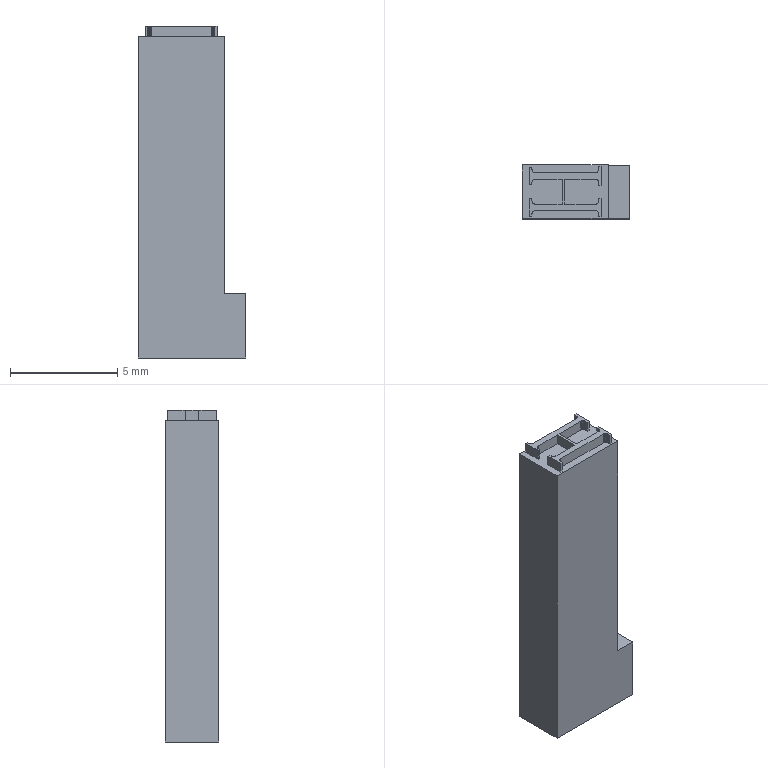Part | NX | features DIE-31 2 | 1 solid | 105 faces | box 5 x 2.5 x 15.5 mm | volume 158.762 mm3 | plane 105